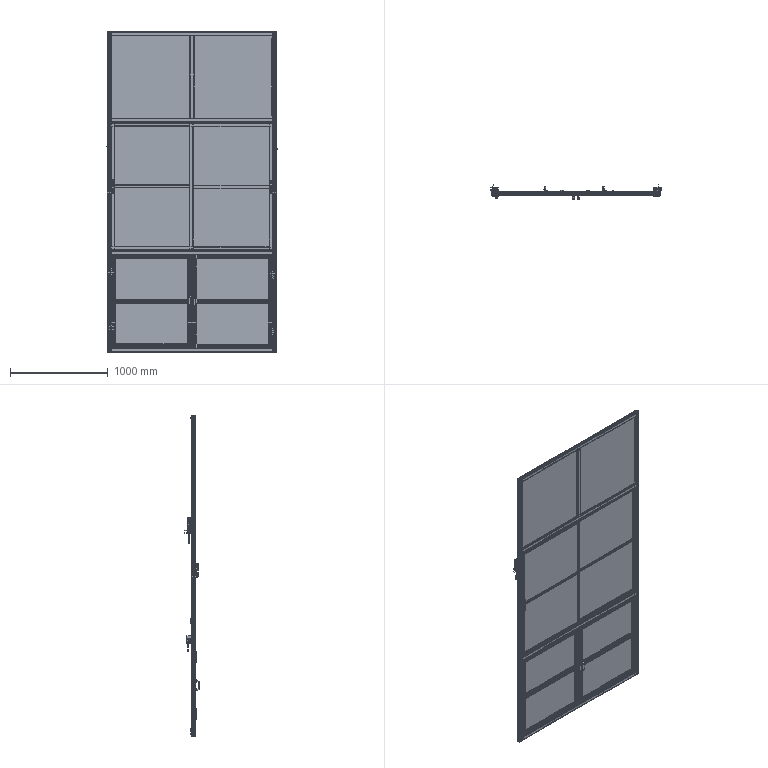Part | SolidWorks | 400 solids | 25380 faces | volume 39443592 mm3 | plane 14439 | cylinder 6143 | cone 2730 | spline 1460 | torus 496 | sphere 112 | commonest cylinder face diameters 1 x506 2 x450 5 x360 2.5 x356 0.562 x300 6.8 x291